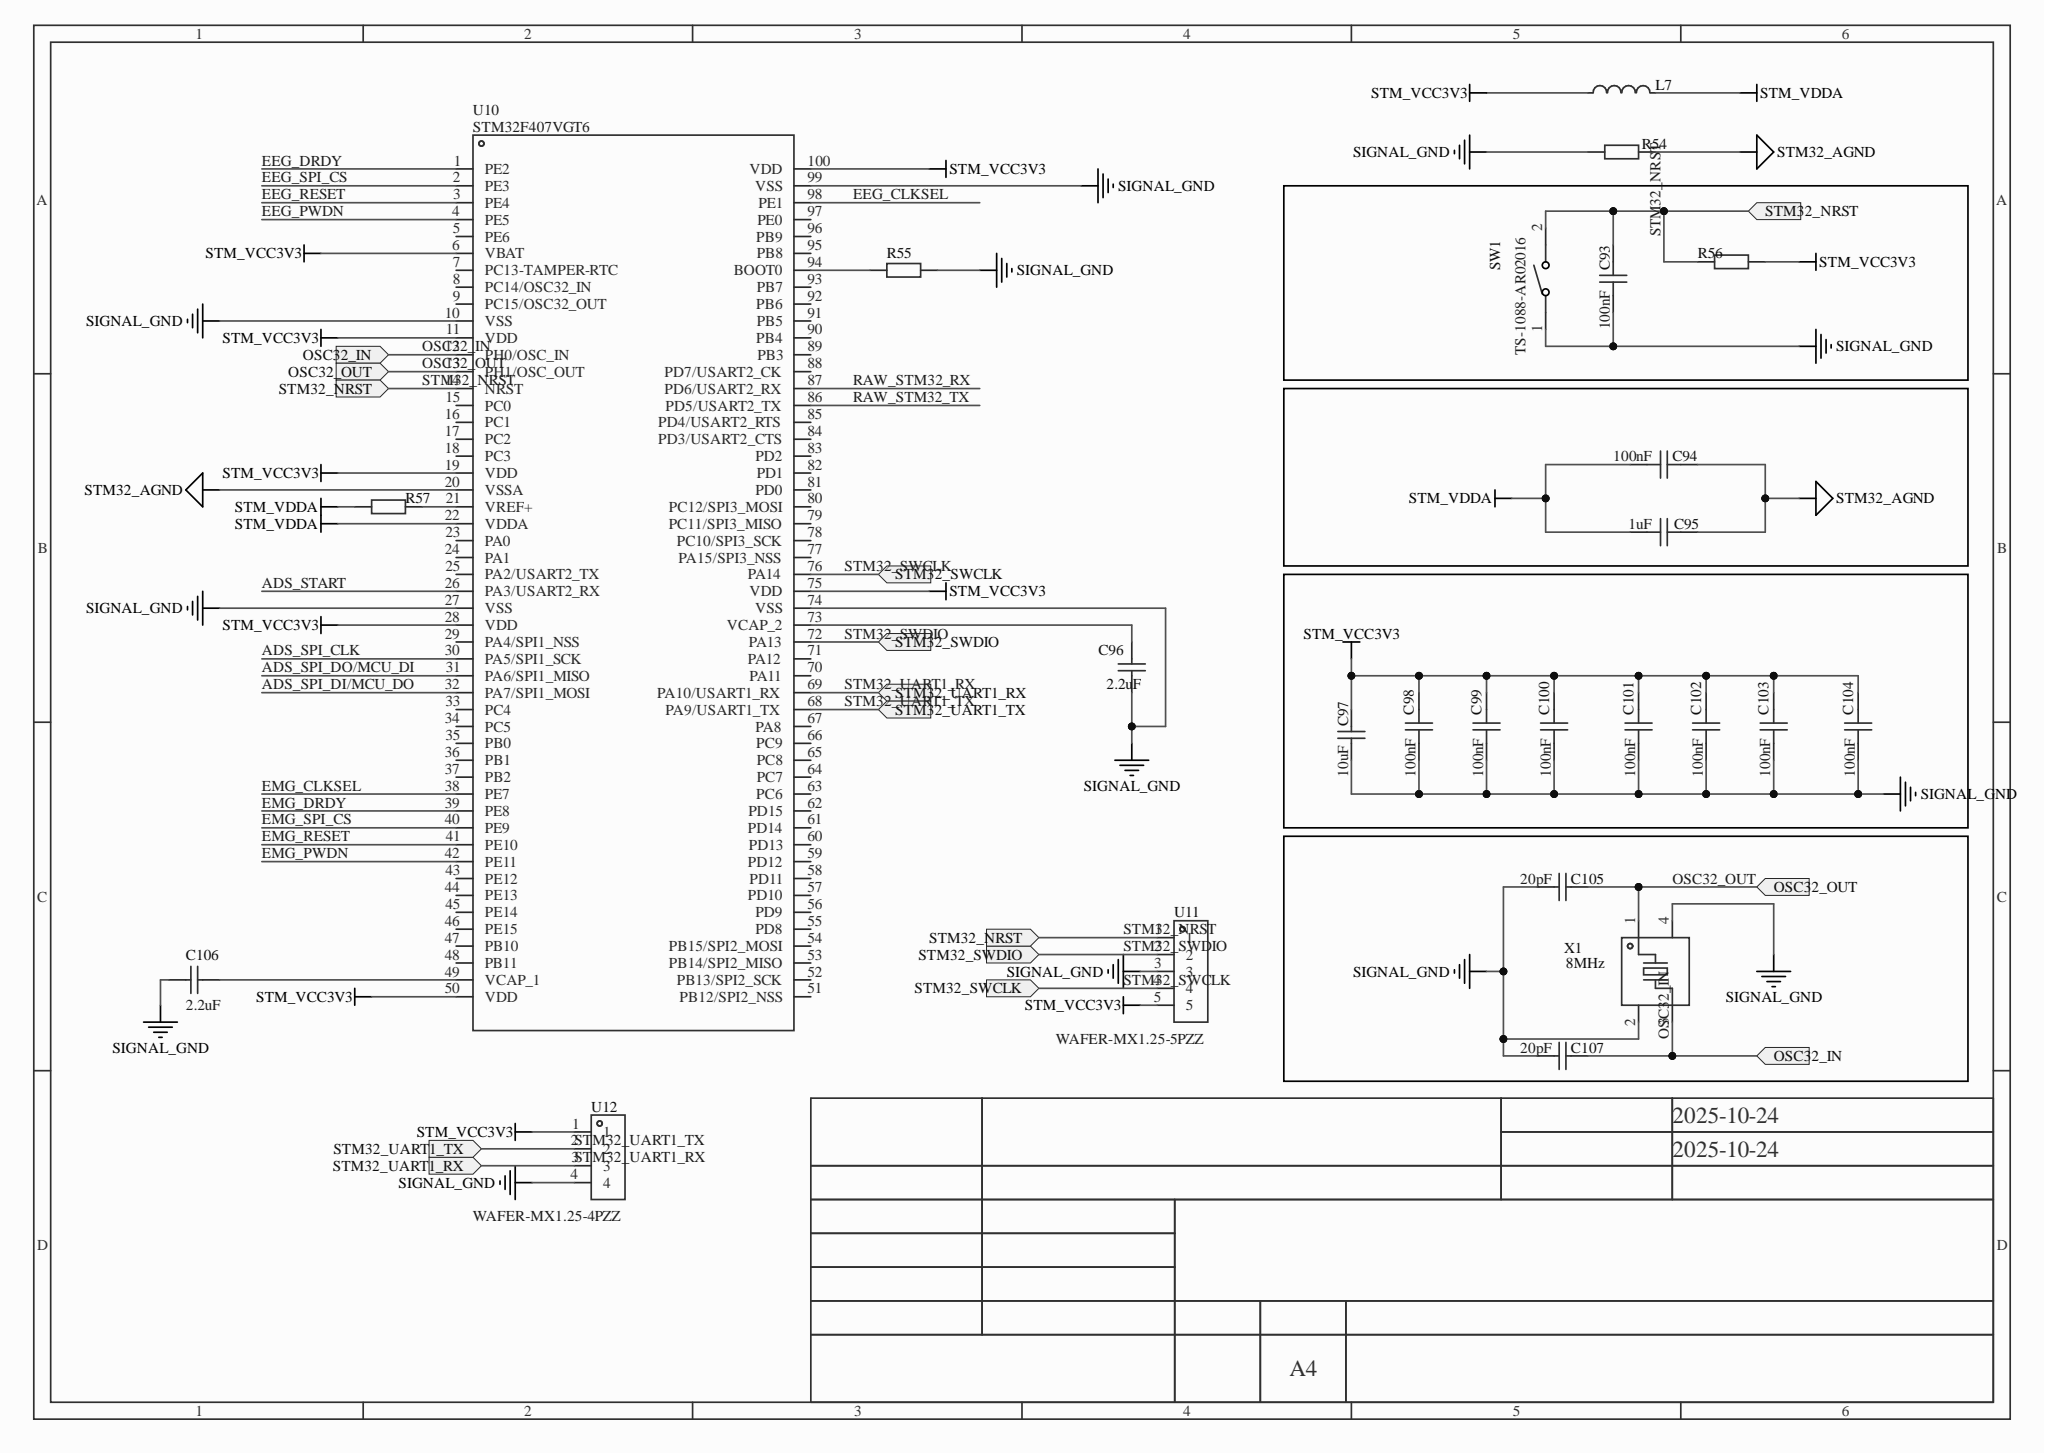Circuit board | Altium Designer | 212 parts | 123 nets | one sheet of the schematic
Parts on this sheet (reference | value | footprint):
C93 | 100nF | C0402
C94 | 100nF | C0402
C95 | 1uF | C0402
C96 | 2.2uF | C0603
C97 | 10uF | C0603
C98 | 100nF | C0402
C99 | 100nF | C0402
C100 | 100nF | C0402
C101 | 100nF | C0402
C102 | 100nF | C0402
C103 | 100nF | C0402
C104 | 100nF | C0402
C105 | 20pF | C0402
C106 | 2.2uF | C0603
C107 | 20pF | C0402
L7 | GZ1608D601TF | L0603
R54 | R0402
R55 | R0402
R56 | R0402
R57 | R0402
SW1 | TS-1088-AR02016 | SW-SMD_L3.9-W3.0-P4.45
U10 | STM32F407VGT6 | LQFP-100_L14.0-W14.0-P0.50-LS16.0-BL
U11 | WAFER-MX1.25-5PZZ | CONN-TH_5P-P1.25_XUNPU_WAFER-MX1.25-5PZZ
U12 | WAFER-MX1.25-4PZZ | CONN-TH_4P-P1.25_WAFER-MX1.25-4PZZ
X1 | 8MHz | CRYSTAL-SMD_4P-L3.2-W2.5-BL
Nets of these parts (net: part-pin ...):
STM_VDDA: C94-2 C95-2 L7-2 R57-1 U10-22
STM_VCC3V3: C97-2 C98-2 C99-2 C100-2 C101-2 C102-2 C103-2 C104-2 L7-1 R56-2 U11-5 U12-1 U10-6 U10-11 U10-19 U10-28 U10-50 U10-75 U10-100
STM32_UART1_TX: U12-2 U10-68
STM32_UART1_RX: U12-3 U10-69
STM32_SWDIO: U11-2 U10-72
STM32_SWCLK: U11-4 U10-76
STM32_NRST: C93-2 R56-1 SW1-2 U11-1 U10-14
STM32_AGND: C94-1 C95-1 R54-2 U10-20
SIGNAL_GND: C93-1 C96-1 C97-1 C98-1 C99-1 C100-1 C101-1 C102-1 C103-1 C104-1 C105-1 C106-2 C107-1 R54-1 R55-2 SW1-1 U11-3 U12-4 X1-2 X1-4 U10-10 U10-27 U10-74 U10-99
RAW_STM32_TX: U10-86
RAW_STM32_RX: U10-87
OSC32_OUT: C105-2 X1-1 U10-13
OSC32_IN: C107-2 X1-3 U10-12
NetR57_2: R57-2 U10-21
NetR55_1: R55-1 U10-94
NetC106_1: C106-1 U10-49
NetC96_2: C96-2 U10-73
EMG_SPI_CS: U10-40
EMG_RESET: U10-41
EMG_PWDN: U10-42
EMG_DRDY: U10-39
EMG_CLKSEL: U10-38
EEG_SPI_CS: U10-2
EEG_RESET: U10-3
EEG_PWDN: U10-4
EEG_DRDY: U10-1
EEG_CLKSEL: U10-98
ADS_START: U10-26
ADS_SPI_DO/MCU_DI: U10-31
ADS_SPI_DI/MCU_DO: U10-32
ADS_SPI_CLK: U10-30